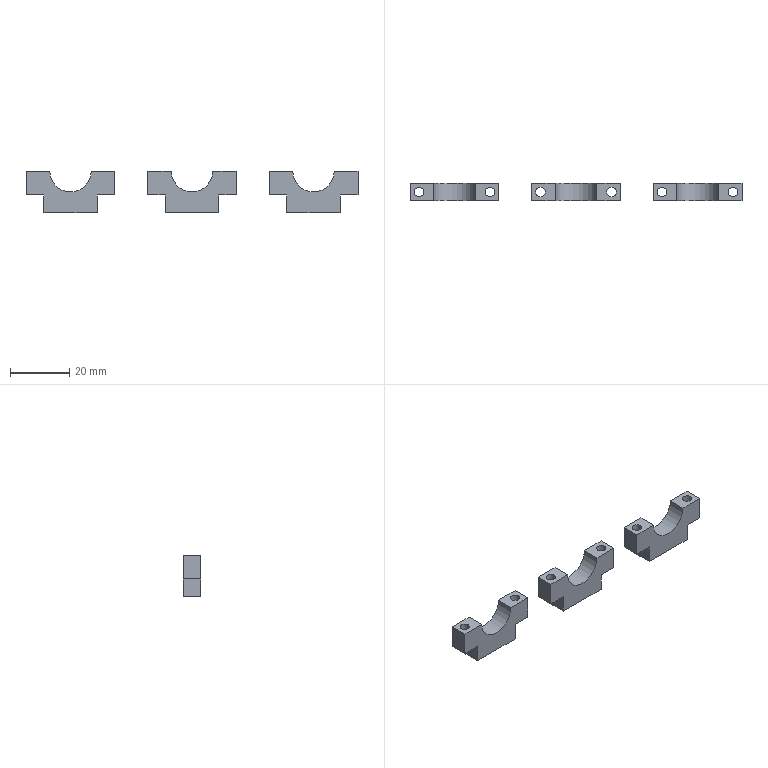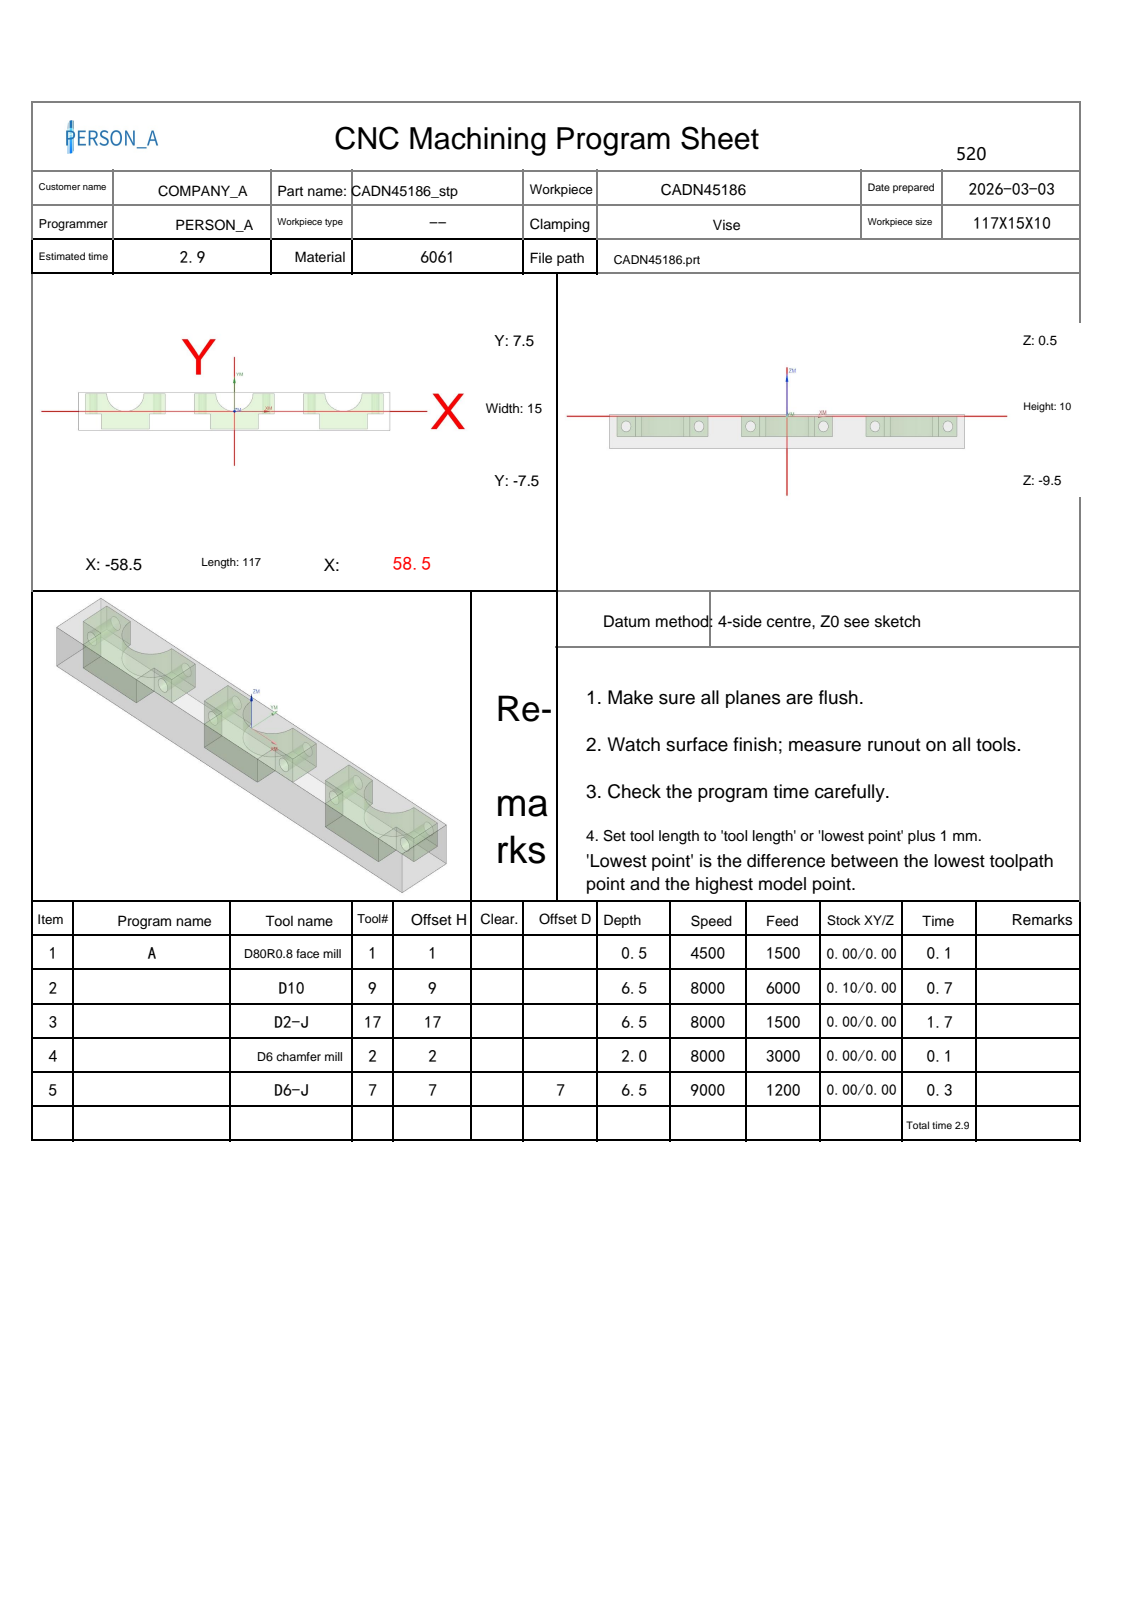NC program | NX | posted by the shop | part box 112 x 6 x 14 mm
Lines 4856 to 5059 of 5059:
N4 T02 M06
(D6 chamfer mill  D=6. R=0. H=02 ce=0.00 di=0.00)
(MAX_Z=50. MIN_Z=-1.5 Time=0.14M)
G00 G90 G54 X-40.75 Y-9.128 M03 S8000
G43 H02 Z50.
M08
Z2.099
G01 Z-1.5 F3000.
G03 X-40.67 Y-8.828 I-.52 J.3
X-40.97 Y-8.308 I-.6 J0.0
G01 X-41. Y-8.3
X-50.
G02 X-51.3 Y-7. I0.0 J1.3
G01 Y-2.3
X-56.
G02 X-57.3 Y-1. I0.0 J1.3
G01 Y7.
G02 X-56. Y8.3 I1.3 J0.0
G01 X-48.
G02 X-46.7 Y7. I0.0 J-1.3
G03 X-41. Y1.3 I5.7 J0.0
X-35.3 Y7. I0.0 J5.7
G02 X-34. Y8.3 I1.3 J0.0
G01 X-26.
G02 X-24.7 Y7. I0.0 J-1.3
G01 Y-1.
G02 X-26. Y-2.3 I-1.3 J0.0
G01 X-30.7
Y-7.
G02 X-32. Y-8.3 I-1.3 J0.0
G01 X-41.
X-41.03 Y-8.308
G03 X-41.33 Y-8.828 I.3 J-.52
X-41.25 Y-9.128 I.6 J0.0
G01 Z2.099
G00 Z50.
X.25
Z2.099
G01 Z-1.5
G03 X.33 Y-8.828 I-.52 J.3
X.03 Y-8.308 I-.6 J0.0
G01 X0.0 Y-8.3
X-9.
G02 X-10.3 Y-7. I0.0 J1.3
G01 Y-2.3
X-15.
G02 X-16.3 Y-1. I0.0 J1.3
G01 Y7.
G02 X-15. Y8.3 I1.3 J0.0
G01 X-7.
G02 X-5.7 Y7. I0.0 J-1.3
G03 X0.0 Y1.3 I5.7 J0.0
X5.7 Y7. I0.0 J5.7
G02 X7. Y8.3 I1.3 J0.0
G01 X15.
G02 X16.3 Y7. I0.0 J-1.3
G01 Y-1.
G02 X15. Y-2.3 I-1.3 J0.0
G01 X10.3
Y-7.
G02 X9. Y-8.3 I-1.3 J0.0
G01 X0.0
X-.03 Y-8.308
G03 X-.33 Y-8.828 I.3 J-.52
X-.25 Y-9.128 I.6 J0.0
G01 Z2.099
G00 Z50.
X41.25
Z2.099
G01 Z-1.5
G03 X41.33 Y-8.828 I-.52 J.3
X41.03 Y-8.308 I-.6 J0.0
G01 X41. Y-8.3
X32.
G02 X30.7 Y-7. I0.0 J1.3
G01 Y-2.3
X26.
G02 X24.7 Y-1. I0.0 J1.3
G01 Y7.
G02 X26. Y8.3 I1.3 J0.0
G01 X34.
G02 X35.3 Y7. I0.0 J-1.3
G03 X41. Y1.3 I5.7 J0.0
X46.7 Y7. I0.0 J5.7
G02 X48. Y8.3 I1.3 J0.0
G01 X56.
G02 X57.3 Y7. I0.0 J-1.3
G01 Y-1.
G02 X56. Y-2.3 I-1.3 J0.0
G01 X51.3
Y-7.
G02 X50. Y-8.3 I-1.3 J0.0
G01 X41.
X40.97 Y-8.308
G03 X40.67 Y-8.828 I.3 J-.52
X40.75 Y-9.128 I.6 J0.0
G01 Z2.099
G00 Z50.
G91 G28 Z0.0
M05
M09
G91 G28 Z0.0
M01
N5 T07 M06
(D6-J  D=6. R=0. H=07 ce=0.00 di=0.00)
(D.N=07 MAX_Z=50. MIN_Z=-6. Time=0.32M)
G00 G90 G54 X51.017 Y-11.073 M03 S9000
G43 H07 Z50.
M08
Z-5.5
G01 Z-6. F1200.
G41 D07
X50.992 Y-10.875
G03 X50. Y-10. I-.992 J-.125
G01 X32.
G02 X29. Y-7. I0.0 J3.
G01 Y-4.
X26.
G02 X23. Y-1. I0.0 J3.
G01 Y7.
G02 X26. Y10. I3. J0.0
G01 X34.
G02 X37. Y7. I0.0 J-3.
G03 X41. Y3. I4. J0.0
X45. Y7. I0.0 J4.
G02 X48. Y10. I3. J0.0
G01 X56.
G02 X59. Y7. I0.0 J-3.
G01 Y-1.
G02 X56. Y-4. I-3. J0.0
G01 X53.
Y-7.
G02 X50. Y-10. I-3. J0.0
G01 X49.5
G03 X48.5 Y-11. I0.0 J-1.
G01 G40 Y-11.2
Z-5.5
G00 Z50.
X10.017 Y-11.073
Z-5.5
G01 Z-6.
G41 D07
X9.992 Y-10.875
G03 X9. Y-10. I-.992 J-.125
G01 X-9.
G02 X-12. Y-7. I0.0 J3.
G01 Y-4.
X-15.
G02 X-18. Y-1. I0.0 J3.
G01 Y7.
G02 X-15. Y10. I3. J0.0
G01 X-7.
G02 X-4. Y7. I0.0 J-3.
G03 X0.0 Y3. I4. J0.0
X4. Y7. I0.0 J4.
G02 X7. Y10. I3. J0.0
G01 X15.
G02 X18. Y7. I0.0 J-3.
G01 Y-1.
G02 X15. Y-4. I-3. J0.0
G01 X12.
Y-7.
G02 X9. Y-10. I-3. J0.0
G01 X8.5
G03 X7.5 Y-11. I0.0 J-1.
G01 G40 Y-11.2
Z-5.5
G00 Z50.
X-30.983 Y-11.073
Z-5.5
G01 Z-6.
G41 D07
X-31.008 Y-10.875
G03 X-32. Y-10. I-.992 J-.125
G01 X-50.
G02 X-53. Y-7. I0.0 J3.
G01 Y-4.
X-56.
G02 X-59. Y-1. I0.0 J3.
G01 Y7.
G02 X-56. Y10. I3. J0.0
G01 X-48.
G02 X-45. Y7. I0.0 J-3.
G03 X-41. Y3. I4. J0.0
X-37. Y7. I0.0 J4.
G02 X-34. Y10. I3. J0.0
G01 X-26.
G02 X-23. Y7. I0.0 J-3.
G01 Y-1.
G02 X-26. Y-4. I-3. J0.0
G01 X-29.
Y-7.
G02 X-32. Y-10. I-3. J0.0
G01 X-32.5
G03 X-33.5 Y-11. I0.0 J-1.
G01 G40 Y-11.2
Z-5.5
G00 Z50.
M05
M09
G91 G28 Z0.0
G91 G28 Y0.0
M30
%